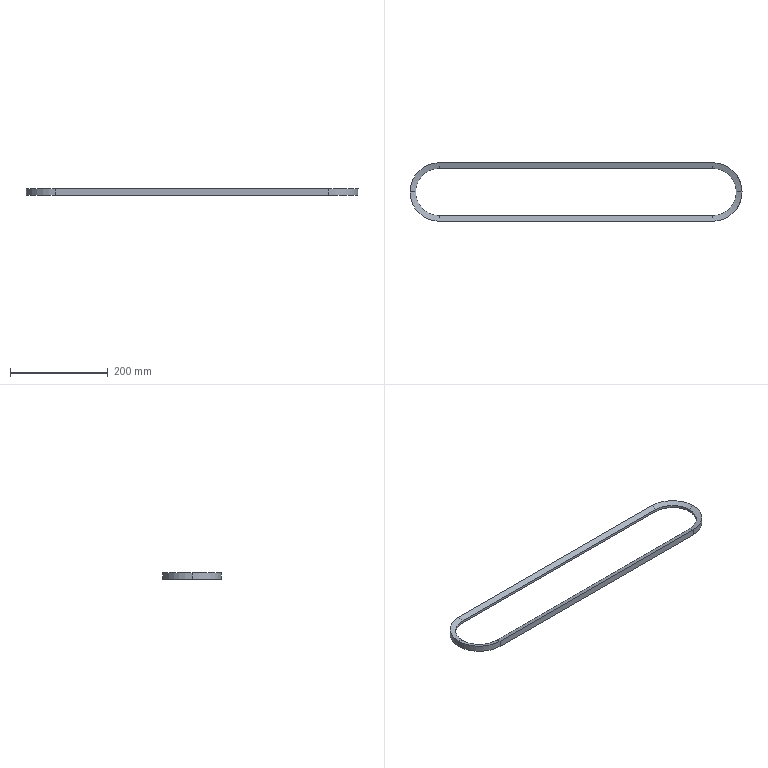Part | SolidWorks | features Sweep 1 | 1 solid | 21 faces | box 680.1 x 120.1 x 13 mm | volume 151786 mm3 | plane 8 | cone 7 | cylinder 6 | commonest cylinder face diameters 97.1 x3 120.1 x3
STEP:
#1=CARTESIAN_POINT('',(280.,48.55,2.5));
#2=VERTEX_POINT('',#1);
#3=CARTESIAN_POINT('',(328.55,0.,2.5));
#4=VERTEX_POINT('',#3);
#5=CARTESIAN_POINT('',(280.,0.,2.5));
#6=DIRECTION('',(0.,0.,-1.));
#7=DIRECTION('',(0.,1.,0.));
#8=AXIS2_PLACEMENT_3D('',#5,#6,#7);
#9=CIRCLE('',#8,48.55);
#10=EDGE_CURVE('',#2,#4,#9,.T.);
#11=ORIENTED_EDGE('',*,*,#10,.T.);
#12=CARTESIAN_POINT('',(340.05,0.,6.5));
#13=VERTEX_POINT('',#12);
#14=CARTESIAN_POINT('',(340.05,0.,6.5));
#15=DIRECTION('',(0.9445,0.,0.3285));
#16=VECTOR('',#15,1000.);
#17=LINE('',#14,#16);
#18=EDGE_CURVE('',#4,#13,#17,.T.);
#19=ORIENTED_EDGE('',*,*,#18,.T.);
#20=CARTESIAN_POINT('',(280.,60.05,6.5));
#21=VERTEX_POINT('',#20);
#22=CARTESIAN_POINT('',(280.,0.,6.5));
#23=DIRECTION('',(0.,0.,-1.));
#24=DIRECTION('',(0.,1.,0.));
#25=AXIS2_PLACEMENT_3D('',#22,#23,#24);
#26=CIRCLE('',#25,60.05);
#27=EDGE_CURVE('',#21,#13,#26,.T.);
#28=ORIENTED_EDGE('',*,*,#27,.F.);
#29=CARTESIAN_POINT('',(280.,60.05,6.5));
#30=DIRECTION('',(0.,-0.9445,-0.3285));
#31=VECTOR('',#30,1000.);
#32=LINE('',#29,#31);
#33=EDGE_CURVE('',#21,#2,#32,.T.);
#34=ORIENTED_EDGE('',*,*,#33,.T.);
#35=EDGE_LOOP('',(#11,#19,#28,#34));
#36=FACE_OUTER_BOUND('',#35,.T.);
#37=CARTESIAN_POINT('',(280.,0.,6.5));
#38=DIRECTION('',(0.,0.,1.));
#39=DIRECTION('',(1.,0.,0.));
#40=AXIS2_PLACEMENT_3D('',#37,#38,#39);
#41=CONICAL_SURFACE('',#40,60.05,1.236);
#42=ADVANCED_FACE('',(#36),#41,.F.);
#43=CARTESIAN_POINT('',(-280.,-60.05,-6.5));
#44=VERTEX_POINT('',#43);
#45=CARTESIAN_POINT('',(-340.05,0.,-6.5));
#46=VERTEX_POINT('',#45);
#47=CARTESIAN_POINT('',(-280.,0.,-6.5));
#48=DIRECTION('',(0.,0.,-1.));
#49=DIRECTION('',(0.,-1.,0.));
#50=AXIS2_PLACEMENT_3D('',#47,#48,#49);
#51=CIRCLE('',#50,60.05);
#52=EDGE_CURVE('',#44,#46,#51,.T.);
#53=ORIENTED_EDGE('',*,*,#52,.F.);
#54=CARTESIAN_POINT('',(-280.,-60.05,6.5));
#55=VERTEX_POINT('',#54);
#56=CARTESIAN_POINT('',(-280.,-60.05,-6.5));
#57=DIRECTION('',(0.,0.,1.));
#58=VECTOR('',#57,1000.);
#59=LINE('',#56,#58);
#60=EDGE_CURVE('',#44,#55,#59,.T.);
#61=ORIENTED_EDGE('',*,*,#60,.T.);
#62=CARTESIAN_POINT('',(-340.05,0.,6.5));
#63=VERTEX_POINT('',#62);
#64=CARTESIAN_POINT('',(-280.,0.,6.5));
#65=DIRECTION('',(0.,0.,-1.));
#66=DIRECTION('',(0.,-1.,0.));
#67=AXIS2_PLACEMENT_3D('',#64,#65,#66);
#68=CIRCLE('',#67,60.05);
#69=EDGE_CURVE('',#55,#63,#68,.T.);
#70=ORIENTED_EDGE('',*,*,#69,.T.);
#71=CARTESIAN_POINT('',(-340.05,0.,-6.5));
#72=DIRECTION('',(0.,0.,1.));
#73=VECTOR('',#72,1000.);
#74=LINE('',#71,#73);
#75=EDGE_CURVE('',#46,#63,#74,.T.);
#76=ORIENTED_EDGE('',*,*,#75,.F.);
#77=EDGE_LOOP('',(#53,#61,#70,#76));
#78=FACE_OUTER_BOUND('',#77,.T.);
#79=CARTESIAN_POINT('',(-280.,0.,0.));
#80=DIRECTION('',(0.,0.,-1.));
#81=DIRECTION('',(-1.,0.,0.));
#82=AXIS2_PLACEMENT_3D('',#79,#80,#81);
#83=CYLINDRICAL_SURFACE('',#82,60.05);
#84=ADVANCED_FACE('',(#78),#83,.T.);
#85=CARTESIAN_POINT('',(-280.,-48.55,-2.5));
#86=VERTEX_POINT('',#85);
#87=CARTESIAN_POINT('',(-328.55,0.,-2.5));
#88=VERTEX_POINT('',#87);
#89=CARTESIAN_POINT('',(-280.,0.,-2.5));
#90=DIRECTION('',(0.,0.,-1.));
#91=DIRECTION('',(0.,-1.,0.));
#92=AXIS2_PLACEMENT_3D('',#89,#90,#91);
#93=CIRCLE('',#92,48.55);
#94=EDGE_CURVE('',#86,#88,#93,.T.);
#95=ORIENTED_EDGE('',*,*,#94,.F.);
#96=CARTESIAN_POINT('',(-280.,-60.05,-6.5));
#97=DIRECTION('',(0.,-0.9445,-0.3285));
#98=VECTOR('',#97,1000.);
#99=LINE('',#96,#98);
#100=EDGE_CURVE('',#86,#44,#99,.T.);
#101=ORIENTED_EDGE('',*,*,#100,.T.);
#102=ORIENTED_EDGE('',*,*,#52,.T.);
#103=CARTESIAN_POINT('',(-340.05,0.,-6.5));
#104=DIRECTION('',(-0.9445,0.,-0.3285));
#105=VECTOR('',#104,1000.);
#106=LINE('',#103,#105);
#107=EDGE_CURVE('',#88,#46,#106,.T.);
#108=ORIENTED_EDGE('',*,*,#107,.F.);
#109=EDGE_LOOP('',(#95,#101,#102,#108));
#110=FACE_OUTER_BOUND('',#109,.T.);
#111=CARTESIAN_POINT('',(-280.,0.,-2.5));
#112=DIRECTION('',(0.,0.,-1.));
#113=DIRECTION('',(-1.,0.,0.));
#114=AXIS2_PLACEMENT_3D('',#111,#112,#113);
#115=CONICAL_SURFACE('',#114,48.55,1.236);
#116=ADVANCED_FACE('',(#110),#115,.F.);
#117=CARTESIAN_POINT('',(-280.,-48.55,2.5));
#118=VERTEX_POINT('',#117);
#119=CARTESIAN_POINT('',(-328.55,0.,2.5));
#120=VERTEX_POINT('',#119);
#121=CARTESIAN_POINT('',(-280.,0.,2.5));
#122=DIRECTION('',(0.,0.,-1.));
#123=DIRECTION('',(0.,-1.,0.));
#124=AXIS2_PLACEMENT_3D('',#121,#122,#123);
#125=CIRCLE('',#124,48.55);
#126=EDGE_CURVE('',#118,#120,#125,.T.);
#127=ORIENTED_EDGE('',*,*,#126,.F.);
#128=CARTESIAN_POINT('',(-280.,-48.55,-2.5));
#129=DIRECTION('',(0.,0.,-1.));
#130=VECTOR('',#129,1000.);
#131=LINE('',#128,#130);
#132=EDGE_CURVE('',#118,#86,#131,.T.);
#133=ORIENTED_EDGE('',*,*,#132,.T.);
#134=ORIENTED_EDGE('',*,*,#94,.T.);
#135=CARTESIAN_POINT('',(-328.55,0.,-2.5));
#136=DIRECTION('',(0.,0.,-1.));
#137=VECTOR('',#136,1000.);
#138=LINE('',#135,#137);
#139=EDGE_CURVE('',#120,#88,#138,.T.);
#140=ORIENTED_EDGE('',*,*,#139,.F.);
#141=EDGE_LOOP('',(#127,#133,#134,#140));
#142=FACE_OUTER_BOUND('',#141,.T.);
#143=CARTESIAN_POINT('',(-280.,0.,0.));
#144=DIRECTION('',(0.,0.,-1.));
#145=DIRECTION('',(-1.,0.,0.));
#146=AXIS2_PLACEMENT_3D('',#143,#144,#145);
#147=CYLINDRICAL_SURFACE('',#146,48.55);
#148=ADVANCED_FACE('',(#142),#147,.F.);
#149=ORIENTED_EDGE('',*,*,#60,.F.);
#150=CARTESIAN_POINT('',(280.,-60.05,-6.5));
#151=VERTEX_POINT('',#150);
#152=CARTESIAN_POINT('',(280.,-60.05,-6.5));
#153=DIRECTION('',(-1.,0.,0.));
#154=VECTOR('',#153,1000.);
#155=LINE('',#152,#154);
#156=EDGE_CURVE('',#151,#44,#155,.T.);
#157=ORIENTED_EDGE('',*,*,#156,.F.);
#158=CARTESIAN_POINT('',(280.,-60.05,6.5));
#159=VERTEX_POINT('',#158);
#160=CARTESIAN_POINT('',(280.,-60.05,-6.5));
#161=DIRECTION('',(0.,0.,1.));
#162=VECTOR('',#161,1000.);
#163=LINE('',#160,#162);
#164=EDGE_CURVE('',#151,#159,#163,.T.);
#165=ORIENTED_EDGE('',*,*,#164,.T.);
#166=CARTESIAN_POINT('',(280.,-60.05,6.5));
#167=DIRECTION('',(-1.,0.,0.));
#168=VECTOR('',#167,1000.);
#169=LINE('',#166,#168);
#170=EDGE_CURVE('',#159,#55,#169,.T.);
#171=ORIENTED_EDGE('',*,*,#170,.T.);
#172=EDGE_LOOP('',(#149,#157,#165,#171));
#173=FACE_OUTER_BOUND('',#172,.T.);
#174=CARTESIAN_POINT('',(280.,-60.05,-6.5));
#175=DIRECTION('',(0.,-1.,0.));
#176=DIRECTION('',(1.,0.,0.));
#177=AXIS2_PLACEMENT_3D('',#174,#175,#176);
#178=PLANE('',#177);
#179=ADVANCED_FACE('',(#173),#178,.T.);
#180=ORIENTED_EDGE('',*,*,#156,.T.);
#181=ORIENTED_EDGE('',*,*,#100,.F.);
#182=CARTESIAN_POINT('',(280.,-48.55,-2.5));
#183=VERTEX_POINT('',#182);
#184=CARTESIAN_POINT('',(280.,-48.55,-2.5));
#185=DIRECTION('',(-1.,0.,0.));
#186=VECTOR('',#185,1000.);
#187=LINE('',#184,#186);
#188=EDGE_CURVE('',#183,#86,#187,.T.);
#189=ORIENTED_EDGE('',*,*,#188,.F.);
#190=CARTESIAN_POINT('',(280.,-60.05,-6.5));
#191=DIRECTION('',(0.,-0.9445,-0.3285));
#192=VECTOR('',#191,1000.);
#193=LINE('',#190,#192);
#194=EDGE_CURVE('',#183,#151,#193,.T.);
#195=ORIENTED_EDGE('',*,*,#194,.T.);
#196=EDGE_LOOP('',(#180,#181,#189,#195));
#197=FACE_OUTER_BOUND('',#196,.T.);
#198=CARTESIAN_POINT('',(280.,-60.05,-6.5));
#199=DIRECTION('',(0.,0.3285,-0.9445));
#200=DIRECTION('',(0.,0.9445,0.3285));
#201=AXIS2_PLACEMENT_3D('',#198,#199,#200);
#202=PLANE('',#201);
#203=ADVANCED_FACE('',(#197),#202,.T.);
#204=ORIENTED_EDGE('',*,*,#188,.T.);
#205=ORIENTED_EDGE('',*,*,#132,.F.);
#206=CARTESIAN_POINT('',(280.,-48.55,2.5));
#207=VERTEX_POINT('',#206);
#208=CARTESIAN_POINT('',(280.,-48.55,2.5));
#209=DIRECTION('',(-1.,0.,0.));
#210=VECTOR('',#209,1000.);
#211=LINE('',#208,#210);
#212=EDGE_CURVE('',#207,#118,#211,.T.);
#213=ORIENTED_EDGE('',*,*,#212,.F.);
#214=CARTESIAN_POINT('',(280.,-48.55,-2.5));
#215=DIRECTION('',(0.,0.,-1.));
#216=VECTOR('',#215,1000.);
#217=LINE('',#214,#216);
#218=EDGE_CURVE('',#207,#183,#217,.T.);
#219=ORIENTED_EDGE('',*,*,#218,.T.);
#220=EDGE_LOOP('',(#204,#205,#213,#219));
#221=FACE_OUTER_BOUND('',#220,.T.);
#222=CARTESIAN_POINT('',(280.,-48.55,-2.5));
#223=DIRECTION('',(0.,1.,0.));
#224=DIRECTION('',(-1.,0.,0.));
#225=AXIS2_PLACEMENT_3D('',#222,#223,#224);
#226=PLANE('',#225);
#227=ADVANCED_FACE('',(#221),#226,.T.);
#228=ORIENTED_EDGE('',*,*,#212,.T.);
#229=CARTESIAN_POINT('',(-280.,-60.05,6.5));
#230=DIRECTION('',(0.,0.9445,-0.3285));
#231=VECTOR('',#230,1000.);
#232=LINE('',#229,#231);
#233=EDGE_CURVE('',#55,#118,#232,.T.);
#234=ORIENTED_EDGE('',*,*,#233,.F.);
#235=ORIENTED_EDGE('',*,*,#170,.F.);
#236=CARTESIAN_POINT('',(280.,-60.05,6.5));
#237=DIRECTION('',(0.,0.9445,-0.3285));
#238=VECTOR('',#237,1000.);
#239=LINE('',#236,#238);
#240=EDGE_CURVE('',#159,#207,#239,.T.);
#241=ORIENTED_EDGE('',*,*,#240,.T.);
#242=EDGE_LOOP('',(#228,#234,#235,#241));
#243=FACE_OUTER_BOUND('',#242,.T.);
#244=CARTESIAN_POINT('',(280.,-60.05,6.5));
#245=DIRECTION('',(0.,0.3285,0.9445));
#246=DIRECTION('',(0.,-0.9445,0.3285));
#247=AXIS2_PLACEMENT_3D('',#244,#245,#246);
#248=PLANE('',#247);
#249=ADVANCED_FACE('',(#243),#248,.T.);
#250=ORIENTED_EDGE('',*,*,#164,.F.);
#251=CARTESIAN_POINT('',(280.,60.05,-6.5));
#252=VERTEX_POINT('',#251);
#253=CARTESIAN_POINT('',(280.,0.,-6.5));
#254=DIRECTION('',(0.,0.,-1.));
#255=DIRECTION('',(0.,1.,0.));
#256=AXIS2_PLACEMENT_3D('',#253,#254,#255);
#257=CIRCLE('',#256,60.05);
#258=EDGE_CURVE('',#252,#151,#257,.T.);
#259=ORIENTED_EDGE('',*,*,#258,.F.);
#260=CARTESIAN_POINT('',(280.,60.05,-6.5));
#261=DIRECTION('',(0.,0.,1.));
#262=VECTOR('',#261,1000.);
#263=LINE('',#260,#262);
#264=EDGE_CURVE('',#252,#21,#263,.T.);
#265=ORIENTED_EDGE('',*,*,#264,.T.);
#266=ORIENTED_EDGE('',*,*,#27,.T.);
#267=CARTESIAN_POINT('',(280.,0.,6.5));
#268=DIRECTION('',(0.,0.,-1.));
#269=DIRECTION('',(0.,1.,0.));
#270=AXIS2_PLACEMENT_3D('',#267,#268,#269);
#271=CIRCLE('',#270,60.05);
#272=EDGE_CURVE('',#13,#159,#271,.T.);
#273=ORIENTED_EDGE('',*,*,#272,.T.);
#274=EDGE_LOOP('',(#250,#259,#265,#266,#273));
#275=FACE_OUTER_BOUND('',#274,.T.);
#276=CARTESIAN_POINT('',(280.,0.,0.));
#277=DIRECTION('',(0.,0.,-1.));
#278=DIRECTION('',(-1.,0.,0.));
#279=AXIS2_PLACEMENT_3D('',#276,#277,#278);
#280=CYLINDRICAL_SURFACE('',#279,60.05);
#281=ADVANCED_FACE('',(#275),#280,.T.);
#282=ORIENTED_EDGE('',*,*,#258,.T.);
#283=ORIENTED_EDGE('',*,*,#194,.F.);
#284=CARTESIAN_POINT('',(280.,48.55,-2.5));
#285=VERTEX_POINT('',#284);
#286=CARTESIAN_POINT('',(280.,0.,-2.5));
#287=DIRECTION('',(0.,0.,-1.));
#288=DIRECTION('',(0.,1.,0.));
#289=AXIS2_PLACEMENT_3D('',#286,#287,#288);
#290=CIRCLE('',#289,48.55);
#291=EDGE_CURVE('',#285,#183,#290,.T.);
#292=ORIENTED_EDGE('',*,*,#291,.F.);
#293=CARTESIAN_POINT('',(280.,60.05,-6.5));
#294=DIRECTION('',(0.,0.9445,-0.3285));
#295=VECTOR('',#294,1000.);
#296=LINE('',#293,#295);
#297=EDGE_CURVE('',#285,#252,#296,.T.);
#298=ORIENTED_EDGE('',*,*,#297,.T.);
#299=EDGE_LOOP('',(#282,#283,#292,#298));
#300=FACE_OUTER_BOUND('',#299,.T.);
#301=CARTESIAN_POINT('',(280.,0.,-2.5));
#302=DIRECTION('',(0.,0.,-1.));
#303=DIRECTION('',(-1.,0.,0.));
#304=AXIS2_PLACEMENT_3D('',#301,#302,#303);
#305=CONICAL_SURFACE('',#304,48.55,1.236);
#306=ADVANCED_FACE('',(#300),#305,.F.);
#307=ORIENTED_EDGE('',*,*,#291,.T.);
#308=ORIENTED_EDGE('',*,*,#218,.F.);
#309=CARTESIAN_POINT('',(280.,0.,2.5));
#310=DIRECTION('',(0.,0.,-1.));
#311=DIRECTION('',(0.,1.,0.));
#312=AXIS2_PLACEMENT_3D('',#309,#310,#311);
#313=CIRCLE('',#312,48.55);
#314=EDGE_CURVE('',#4,#207,#313,.T.);
#315=ORIENTED_EDGE('',*,*,#314,.F.);
#316=ORIENTED_EDGE('',*,*,#10,.F.);
#317=CARTESIAN_POINT('',(280.,48.55,-2.5));
#318=DIRECTION('',(0.,0.,-1.));
#319=VECTOR('',#318,1000.);
#320=LINE('',#317,#319);
#321=EDGE_CURVE('',#2,#285,#320,.T.);
#322=ORIENTED_EDGE('',*,*,#321,.T.);
#323=EDGE_LOOP('',(#307,#308,#315,#316,#322));
#324=FACE_OUTER_BOUND('',#323,.T.);
#325=CARTESIAN_POINT('',(280.,0.,0.));
#326=DIRECTION('',(0.,0.,-1.));
#327=DIRECTION('',(-1.,0.,0.));
#328=AXIS2_PLACEMENT_3D('',#325,#326,#327);
#329=CYLINDRICAL_SURFACE('',#328,48.55);
#330=ADVANCED_FACE('',(#324),#329,.F.);
#331=ORIENTED_EDGE('',*,*,#18,.F.);
#332=ORIENTED_EDGE('',*,*,#314,.T.);
#333=ORIENTED_EDGE('',*,*,#240,.F.);
#334=ORIENTED_EDGE('',*,*,#272,.F.);
#335=EDGE_LOOP('',(#331,#332,#333,#334));
#336=FACE_OUTER_BOUND('',#335,.T.);
#337=CARTESIAN_POINT('',(280.,0.,6.5));
#338=DIRECTION('',(0.,0.,1.));
#339=DIRECTION('',(1.,0.,0.));
#340=AXIS2_PLACEMENT_3D('',#337,#338,#339);
#341=CONICAL_SURFACE('',#340,60.05,1.236);
#342=ADVANCED_FACE('',(#336),#341,.F.);
#343=ORIENTED_EDGE('',*,*,#264,.F.);
#344=CARTESIAN_POINT('',(-280.,60.05,-6.5));
#345=VERTEX_POINT('',#344);
#346=CARTESIAN_POINT('',(-280.,60.05,-6.5));
#347=DIRECTION('',(1.,0.,0.));
#348=VECTOR('',#347,1000.);
#349=LINE('',#346,#348);
#350=EDGE_CURVE('',#345,#252,#349,.T.);
#351=ORIENTED_EDGE('',*,*,#350,.F.);
#352=CARTESIAN_POINT('',(-280.,60.05,6.5));
#353=VERTEX_POINT('',#352);
#354=CARTESIAN_POINT('',(-280.,60.05,-6.5));
#355=DIRECTION('',(0.,0.,1.));
#356=VECTOR('',#355,1000.);
#357=LINE('',#354,#356);
#358=EDGE_CURVE('',#345,#353,#357,.T.);
#359=ORIENTED_EDGE('',*,*,#358,.T.);
#360=CARTESIAN_POINT('',(-280.,60.05,6.5));
#361=DIRECTION('',(1.,0.,0.));
#362=VECTOR('',#361,1000.);
#363=LINE('',#360,#362);
#364=EDGE_CURVE('',#353,#21,#363,.T.);
#365=ORIENTED_EDGE('',*,*,#364,.T.);
#366=EDGE_LOOP('',(#343,#351,#359,#365));
#367=FACE_OUTER_BOUND('',#366,.T.);
#368=CARTESIAN_POINT('',(-280.,60.05,-6.5));
#369=DIRECTION('',(0.,1.,0.));
#370=DIRECTION('',(-1.,0.,0.));
#371=AXIS2_PLACEMENT_3D('',#368,#369,#370);
#372=PLANE('',#371);
#373=ADVANCED_FACE('',(#367),#372,.T.);
#374=ORIENTED_EDGE('',*,*,#350,.T.);
#375=ORIENTED_EDGE('',*,*,#297,.F.);
#376=CARTESIAN_POINT('',(-280.,48.55,-2.5));
#377=VERTEX_POINT('',#376);
#378=CARTESIAN_POINT('',(-280.,48.55,-2.5));
#379=DIRECTION('',(1.,0.,0.));
#380=VECTOR('',#379,1000.);
#381=LINE('',#378,#380);
#382=EDGE_CURVE('',#377,#285,#381,.T.);
#383=ORIENTED_EDGE('',*,*,#382,.F.);
#384=CARTESIAN_POINT('',(-280.,60.05,-6.5));
#385=DIRECTION('',(0.,0.9445,-0.3285));
#386=VECTOR('',#385,1000.);
#387=LINE('',#384,#386);
#388=EDGE_CURVE('',#377,#345,#387,.T.);
#389=ORIENTED_EDGE('',*,*,#388,.T.);
#390=EDGE_LOOP('',(#374,#375,#383,#389));
#391=FACE_OUTER_BOUND('',#390,.T.);
#392=CARTESIAN_POINT('',(-280.,60.05,-6.5));
#393=DIRECTION('',(0.,-0.3285,-0.9445));
#394=DIRECTION('',(0.,0.9445,-0.3285));
#395=AXIS2_PLACEMENT_3D('',#392,#393,#394);
#396=PLANE('',#395);
#397=ADVANCED_FACE('',(#391),#396,.T.);
#398=ORIENTED_EDGE('',*,*,#382,.T.);
#399=ORIENTED_EDGE('',*,*,#321,.F.);
#400=CARTESIAN_POINT('',(-280.,48.55,2.5));
#401=VERTEX_POINT('',#400);
#402=CARTESIAN_POINT('',(-280.,48.55,2.5));
#403=DIRECTION('',(1.,0.,0.));
#404=VECTOR('',#403,1000.);
#405=LINE('',#402,#404);
#406=EDGE_CURVE('',#401,#2,#405,.T.);
#407=ORIENTED_EDGE('',*,*,#406,.F.);
#408=CARTESIAN_POINT('',(-280.,48.55,-2.5));
#409=DIRECTION('',(0.,0.,-1.));
#410=VECTOR('',#409,1000.);
#411=LINE('',#408,#410);
#412=EDGE_CURVE('',#401,#377,#411,.T.);
#413=ORIENTED_EDGE('',*,*,#412,.T.);
#414=EDGE_LOOP('',(#398,#399,#407,#413));
#415=FACE_OUTER_BOUND('',#414,.T.);
#416=CARTESIAN_POINT('',(-280.,48.55,-2.5));
#417=DIRECTION('',(0.,-1.,0.));
#418=DIRECTION('',(1.,0.,0.));
#419=AXIS2_PLACEMENT_3D('',#416,#417,#418);
#420=PLANE('',#419);
#421=ADVANCED_FACE('',(#415),#420,.T.);
#422=ORIENTED_EDGE('',*,*,#406,.T.);
#423=ORIENTED_EDGE('',*,*,#33,.F.);
#424=ORIENTED_EDGE('',*,*,#364,.F.);
#425=CARTESIAN_POINT('',(-280.,60.05,6.5));
#426=DIRECTION('',(0.,-0.9445,-0.3285));
#427=VECTOR('',#426,1000.);
#428=LINE('',#425,#427);
#429=EDGE_CURVE('',#353,#401,#428,.T.);
#430=ORIENTED_EDGE('',*,*,#429,.T.);
#431=EDGE_LOOP('',(#422,#423,#424,#430));
#432=FACE_OUTER_BOUND('',#431,.T.);
#433=CARTESIAN_POINT('',(-280.,60.05,6.5));
#434=DIRECTION('',(0.,-0.3285,0.9445));
#435=DIRECTION('',(0.,-0.9445,-0.3285));
#436=AXIS2_PLACEMENT_3D('',#433,#434,#435);
#437=PLANE('',#436);
#438=ADVANCED_FACE('',(#432),#437,.T.);
#439=ORIENTED_EDGE('',*,*,#358,.F.);
#440=CARTESIAN_POINT('',(-280.,0.,-6.5));
#441=DIRECTION('',(0.,0.,-1.));
#442=DIRECTION('',(-1.,0.,0.));
#443=AXIS2_PLACEMENT_3D('',#440,#441,#442);
#444=CIRCLE('',#443,60.05);
#445=EDGE_CURVE('',#46,#345,#444,.T.);
#446=ORIENTED_EDGE('',*,*,#445,.F.);
#447=ORIENTED_EDGE('',*,*,#75,.T.);
#448=CARTESIAN_POINT('',(-280.,0.,6.5));
#449=DIRECTION('',(0.,0.,-1.));
#450=DIRECTION('',(-1.,0.,0.));
#451=AXIS2_PLACEMENT_3D('',#448,#449,#450);
#452=CIRCLE('',#451,60.05);
#453=EDGE_CURVE('',#63,#353,#452,.T.);
#454=ORIENTED_EDGE('',*,*,#453,.T.);
#455=EDGE_LOOP('',(#439,#446,#447,#454));
#456=FACE_OUTER_BOUND('',#455,.T.);
#457=CARTESIAN_POINT('',(-280.,0.,0.));
#458=DIRECTION('',(0.,0.,-1.));
#459=DIRECTION('',(-1.,0.,0.));
#460=AXIS2_PLACEMENT_3D('',#457,#458,#459);
#461=CYLINDRICAL_SURFACE('',#460,60.05);
#462=ADVANCED_FACE('',(#456),#461,.T.);
#463=ORIENTED_EDGE('',*,*,#445,.T.);
#464=ORIENTED_EDGE('',*,*,#388,.F.);
#465=CARTESIAN_POINT('',(-280.,0.,-2.5));
#466=DIRECTION('',(0.,0.,-1.));
#467=DIRECTION('',(-1.,0.,0.));
#468=AXIS2_PLACEMENT_3D('',#465,#466,#467);
#469=CIRCLE('',#468,48.55);
#470=EDGE_CURVE('',#88,#377,#469,.T.);
#471=ORIENTED_EDGE('',*,*,#470,.F.);
#472=ORIENTED_EDGE('',*,*,#107,.T.);
#473=EDGE_LOOP('',(#463,#464,#471,#472));
#474=FACE_OUTER_BOUND('',#473,.T.);
#475=CARTESIAN_POINT('',(-280.,0.,-2.5));
#476=DIRECTION('',(0.,0.,-1.));
#477=DIRECTION('',(-1.,0.,0.));
#478=AXIS2_PLACEMENT_3D('',#475,#476,#477);
#479=CONICAL_SURFACE('',#478,48.55,1.236);
#480=ADVANCED_FACE('',(#474),#479,.F.);
#481=ORIENTED_EDGE('',*,*,#470,.T.);
#482=ORIENTED_EDGE('',*,*,#412,.F.);
#483=CARTESIAN_POINT('',(-280.,0.,2.5));
#484=DIRECTION('',(0.,0.,-1.));
#485=DIRECTION('',(-1.,0.,0.));
#486=AXIS2_PLACEMENT_3D('',#483,#484,#485);
#487=CIRCLE('',#486,48.55);
#488=EDGE_CURVE('',#120,#401,#487,.T.);
#489=ORIENTED_EDGE('',*,*,#488,.F.);
#490=ORIENTED_EDGE('',*,*,#139,.T.);
#491=EDGE_LOOP('',(#481,#482,#489,#490));
#492=FACE_OUTER_BOUND('',#491,.T.);
#493=CARTESIAN_POINT('',(-280.,0.,0.));
#494=DIRECTION('',(0.,0.,-1.));
#495=DIRECTION('',(-1.,0.,0.));
#496=AXIS2_PLACEMENT_3D('',#493,#494,#495);
#497=CYLINDRICAL_SURFACE('',#496,48.55);
#498=ADVANCED_FACE('',(#492),#497,.F.);
#499=ORIENTED_EDGE('',*,*,#488,.T.);
#500=ORIENTED_EDGE('',*,*,#429,.F.);
#501=ORIENTED_EDGE('',*,*,#453,.F.);
#502=CARTESIAN_POINT('',(-340.05,0.,6.5));
#503=DIRECTION('',(0.9445,0.,-0.3285));
#504=VECTOR('',#503,1000.);
#505=LINE('',#502,#504);
#506=EDGE_CURVE('',#63,#120,#505,.T.);
#507=ORIENTED_EDGE('',*,*,#506,.T.);
#508=EDGE_LOOP('',(#499,#500,#501,#507));
#509=FACE_OUTER_BOUND('',#508,.T.);
#510=CARTESIAN_POINT('',(-280.,0.,6.5));
#511=DIRECTION('',(0.,0.,1.));
#512=DIRECTION('',(1.,0.,0.));
#513=AXIS2_PLACEMENT_3D('',#510,#511,#512);
#514=CONICAL_SURFACE('',#513,60.05,1.236);
#515=ADVANCED_FACE('',(#509),#514,.F.);
#516=ORIENTED_EDGE('',*,*,#233,.T.);
#517=ORIENTED_EDGE('',*,*,#126,.T.);
#518=ORIENTED_EDGE('',*,*,#506,.F.);
#519=ORIENTED_EDGE('',*,*,#69,.F.);
#520=EDGE_LOOP('',(#516,#517,#518,#519));
#521=FACE_OUTER_BOUND('',#520,.T.);
#522=CARTESIAN_POINT('',(-280.,0.,6.5));
#523=DIRECTION('',(0.,0.,1.));
#524=DIRECTION('',(1.,0.,0.));
#525=AXIS2_PLACEMENT_3D('',#522,#523,#524);
#526=CONICAL_SURFACE('',#525,60.05,1.236);
#527=ADVANCED_FACE('',(#521),#526,.F.);
#528=CLOSED_SHELL('',(#42,#84,#116,#148,#179,#203,#227,#249,#281,#306,#330,#342,#373,#397,#421,#438,#462,#480,#498,#515,#527));
#529=MANIFOLD_SOLID_BREP('',#528);
#530=CARTESIAN_POINT('',(0.,0.,0.));
#531=DIRECTION('',(0.,0.,1.));
#532=DIRECTION('',(1.,0.,0.));
#533=AXIS2_PLACEMENT_3D('',#530,#531,#532);
#534=(LENGTH_UNIT()NAMED_UNIT(*)SI_UNIT(.MILLI.,.METRE.));
#535=UNCERTAINTY_MEASURE_WITH_UNIT(LENGTH_MEASURE(0.00001),#534,'','');
#536=(NAMED_UNIT(*)PLANE_ANGLE_UNIT()SI_UNIT($,.RADIAN.));
#537=(NAMED_UNIT(*)SI_UNIT($,.STERADIAN.)SOLID_ANGLE_UNIT());
#538=(GEOMETRIC_REPRESENTATION_CONTEXT(3)GLOBAL_UNCERTAINTY_ASSIGNED_CONTEXT((#535))GLOBAL_UNIT_ASSIGNED_CONTEXT((#534,#536,#537))REPRESENTATION_CONTEXT('',''));
#539=ADVANCED_BREP_SHAPE_REPRESENTATION('',(#529,#533),#538);